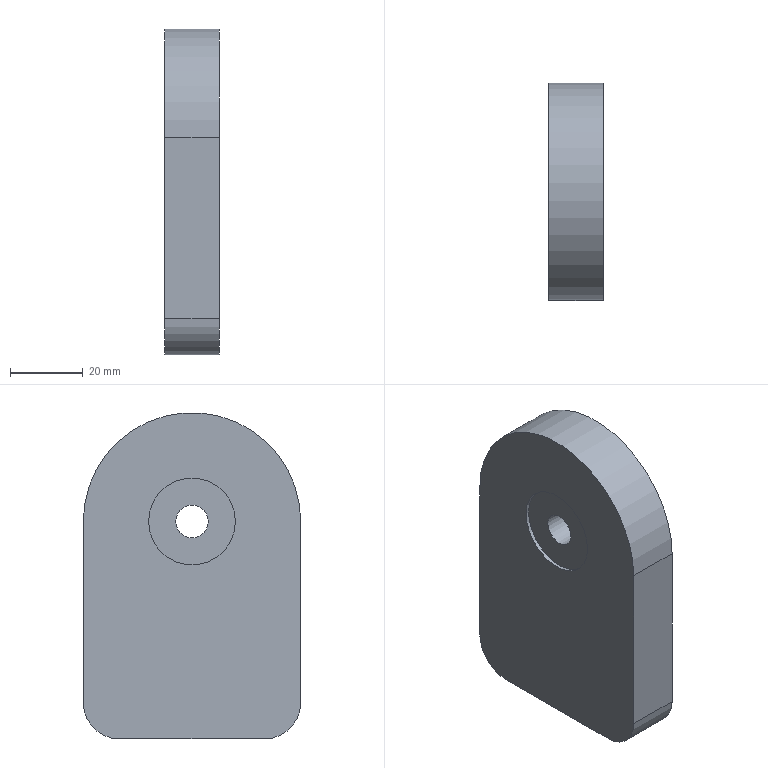Part | STEP file | Frame_lock | 1 solid | 11 faces | box 15 x 60 x 90 mm | volume 73219 mm3 | plane 6 | cylinder 5 | commonest cylinder face diameters 20 x2 9 x1 24 x1 60 x1
STEP:
#1=CARTESIAN_POINT('',(0.,0.,0.));
#2=DIRECTION('',(0.,0.,1.));
#3=DIRECTION('',(1.,0.,0.));
#4=AXIS2_PLACEMENT_3D('',#1,#2,#3);
#5=CARTESIAN_POINT('',(0.,30.,0.));
#6=VERTEX_POINT('',#5);
#7=CARTESIAN_POINT('',(0.,-30.,0.));
#8=VERTEX_POINT('',#7);
#9=CARTESIAN_POINT('',(0.,0.,0.));
#10=DIRECTION('',(1.,0.,0.));
#11=DIRECTION('',(0.,1.,0.));
#12=AXIS2_PLACEMENT_3D('',#9,#10,#11);
#13=CIRCLE('',#12,30.);
#14=CARTESIAN_POINT('',(0.,0.,0.));
#15=DIRECTION('',(-1.,0.,0.));
#16=DIRECTION('',(0.,1.,0.));
#17=AXIS2_PLACEMENT_3D('',#14,#15,#16);
#18=CYLINDRICAL_SURFACE('',#17,30.);
#19=CARTESIAN_POINT('',(6.283,0.));
#20=DIRECTION('',(-1.,0.));
#21=VECTOR('',#20,1.);
#22=LINE('',#19,#21);
#23=(GEOMETRIC_REPRESENTATION_CONTEXT(2)PARAMETRIC_REPRESENTATION_CONTEXT()REPRESENTATION_CONTEXT('',''));
#24=DEFINITIONAL_REPRESENTATION('',(#22),#23);
#25=PCURVE('',#18,#24);
#26=CARTESIAN_POINT('',(0.,0.,-17.885));
#27=DIRECTION('',(1.,0.,0.));
#28=DIRECTION('',(0.,0.,1.));
#29=AXIS2_PLACEMENT_3D('',#26,#27,#28);
#30=PLANE('',#29);
#31=CARTESIAN_POINT('',(17.885,0.));
#32=DIRECTION('',(0.,-1.));
#33=AXIS2_PLACEMENT_2D('',#31,#32);
#34=CIRCLE('',#33,30.);
#35=(GEOMETRIC_REPRESENTATION_CONTEXT(2)PARAMETRIC_REPRESENTATION_CONTEXT()REPRESENTATION_CONTEXT('',''));
#36=DEFINITIONAL_REPRESENTATION('',(#34),#35);
#37=PCURVE('',#30,#36);
#38=SURFACE_CURVE('',#13,(#25,#37),.PCURVE_S1.);
#39=EDGE_CURVE('',#6,#8,#38,.T.);
#40=ORIENTED_EDGE('',*,*,#39,.T.);
#41=CARTESIAN_POINT('',(15.,-30.,0.));
#42=VERTEX_POINT('',#41);
#43=CARTESIAN_POINT('',(0.,-30.,0.));
#44=DIRECTION('',(1.,0.,0.));
#45=VECTOR('',#44,1.);
#46=LINE('',#43,#45);
#47=CARTESIAN_POINT('',(3.142,0.));
#48=DIRECTION('',(0.,-1.));
#49=VECTOR('',#48,1.);
#50=LINE('',#47,#49);
#51=(GEOMETRIC_REPRESENTATION_CONTEXT(2)PARAMETRIC_REPRESENTATION_CONTEXT()REPRESENTATION_CONTEXT('',''));
#52=DEFINITIONAL_REPRESENTATION('',(#50),#51);
#53=PCURVE('',#18,#52);
#54=CARTESIAN_POINT('',(0.,-30.,0.));
#55=DIRECTION('',(0.,1.,0.));
#56=DIRECTION('',(0.,0.,-1.));
#57=AXIS2_PLACEMENT_3D('',#54,#55,#56);
#58=PLANE('',#57);
#59=CARTESIAN_POINT('',(0.,0.));
#60=DIRECTION('',(0.,-1.));
#61=VECTOR('',#60,1.);
#62=LINE('',#59,#61);
#63=(GEOMETRIC_REPRESENTATION_CONTEXT(2)PARAMETRIC_REPRESENTATION_CONTEXT()REPRESENTATION_CONTEXT('',''));
#64=DEFINITIONAL_REPRESENTATION('',(#62),#63);
#65=PCURVE('',#58,#64);
#66=SURFACE_CURVE('',#46,(#53,#65),.PCURVE_S1.);
#67=EDGE_CURVE('',#8,#42,#66,.T.);
#68=ORIENTED_EDGE('',*,*,#67,.T.);
#69=CARTESIAN_POINT('',(15.,30.,0.));
#70=VERTEX_POINT('',#69);
#71=CARTESIAN_POINT('',(15.,0.,0.));
#72=DIRECTION('',(1.,0.,0.));
#73=DIRECTION('',(0.,1.,0.));
#74=AXIS2_PLACEMENT_3D('',#71,#72,#73);
#75=CIRCLE('',#74,30.);
#76=CARTESIAN_POINT('',(6.283,-15.));
#77=DIRECTION('',(-1.,0.));
#78=VECTOR('',#77,1.);
#79=LINE('',#76,#78);
#80=(GEOMETRIC_REPRESENTATION_CONTEXT(2)PARAMETRIC_REPRESENTATION_CONTEXT()REPRESENTATION_CONTEXT('',''));
#81=DEFINITIONAL_REPRESENTATION('',(#79),#80);
#82=PCURVE('',#18,#81);
#83=CARTESIAN_POINT('',(15.,0.,-17.885));
#84=DIRECTION('',(1.,0.,0.));
#85=DIRECTION('',(0.,0.,1.));
#86=AXIS2_PLACEMENT_3D('',#83,#84,#85);
#87=PLANE('',#86);
#88=CARTESIAN_POINT('',(17.885,0.));
#89=DIRECTION('',(0.,-1.));
#90=AXIS2_PLACEMENT_2D('',#88,#89);
#91=CIRCLE('',#90,30.);
#92=(GEOMETRIC_REPRESENTATION_CONTEXT(2)PARAMETRIC_REPRESENTATION_CONTEXT()REPRESENTATION_CONTEXT('',''));
#93=DEFINITIONAL_REPRESENTATION('',(#91),#92);
#94=PCURVE('',#87,#93);
#95=SURFACE_CURVE('',#75,(#82,#94),.PCURVE_S1.);
#96=EDGE_CURVE('',#70,#42,#95,.T.);
#97=ORIENTED_EDGE('',*,*,#96,.F.);
#98=CARTESIAN_POINT('',(0.,30.,0.));
#99=DIRECTION('',(1.,0.,0.));
#100=VECTOR('',#99,1.);
#101=LINE('',#98,#100);
#102=CARTESIAN_POINT('',(6.283,0.));
#103=DIRECTION('',(0.,-1.));
#104=VECTOR('',#103,1.);
#105=LINE('',#102,#104);
#106=(GEOMETRIC_REPRESENTATION_CONTEXT(2)PARAMETRIC_REPRESENTATION_CONTEXT()REPRESENTATION_CONTEXT('',''));
#107=DEFINITIONAL_REPRESENTATION('',(#105),#106);
#108=PCURVE('',#18,#107);
#109=CARTESIAN_POINT('',(0.,30.,-50.));
#110=DIRECTION('',(0.,-1.,0.));
#111=DIRECTION('',(0.,0.,1.));
#112=AXIS2_PLACEMENT_3D('',#109,#110,#111);
#113=PLANE('',#112);
#114=CARTESIAN_POINT('',(50.,0.));
#115=DIRECTION('',(0.,-1.));
#116=VECTOR('',#115,1.);
#117=LINE('',#114,#116);
#118=(GEOMETRIC_REPRESENTATION_CONTEXT(2)PARAMETRIC_REPRESENTATION_CONTEXT()REPRESENTATION_CONTEXT('',''));
#119=DEFINITIONAL_REPRESENTATION('',(#117),#118);
#120=PCURVE('',#113,#119);
#121=SURFACE_CURVE('',#101,(#108,#120),.PCURVE_S1.);
#122=EDGE_CURVE('',#6,#70,#121,.T.);
#123=ORIENTED_EDGE('',*,*,#122,.F.);
#124=EDGE_LOOP('',(#40,#68,#97,#123));
#125=FACE_BOUND('',#124,.T.);
#126=ADVANCED_FACE('',(#125),#18,.T.);
#127=CARTESIAN_POINT('',(0.,30.,-50.));
#128=VERTEX_POINT('',#127);
#129=CARTESIAN_POINT('',(15.,30.,-50.));
#130=VERTEX_POINT('',#129);
#131=CARTESIAN_POINT('',(0.,30.,-50.));
#132=DIRECTION('',(1.,0.,0.));
#133=VECTOR('',#132,1.);
#134=LINE('',#131,#133);
#135=CARTESIAN_POINT('',(0.,0.));
#136=DIRECTION('',(0.,-1.));
#137=VECTOR('',#136,1.);
#138=LINE('',#135,#137);
#139=(GEOMETRIC_REPRESENTATION_CONTEXT(2)PARAMETRIC_REPRESENTATION_CONTEXT()REPRESENTATION_CONTEXT('',''));
#140=DEFINITIONAL_REPRESENTATION('',(#138),#139);
#141=PCURVE('',#113,#140);
#142=CARTESIAN_POINT('',(0.,20.,-50.));
#143=DIRECTION('',(-1.,0.,0.));
#144=DIRECTION('',(0.,1.,0.));
#145=AXIS2_PLACEMENT_3D('',#142,#143,#144);
#146=CYLINDRICAL_SURFACE('',#145,10.);
#147=CARTESIAN_POINT('',(0.,0.));
#148=DIRECTION('',(0.,-1.));
#149=VECTOR('',#148,1.);
#150=LINE('',#147,#149);
#151=(GEOMETRIC_REPRESENTATION_CONTEXT(2)PARAMETRIC_REPRESENTATION_CONTEXT()REPRESENTATION_CONTEXT('',''));
#152=DEFINITIONAL_REPRESENTATION('',(#150),#151);
#153=PCURVE('',#146,#152);
#154=SURFACE_CURVE('',#134,(#141,#153),.PCURVE_S1.);
#155=EDGE_CURVE('',#128,#130,#154,.T.);
#156=ORIENTED_EDGE('',*,*,#155,.T.);
#157=CARTESIAN_POINT('',(15.,30.,-50.));
#158=DIRECTION('',(0.,0.,1.));
#159=VECTOR('',#158,1.);
#160=LINE('',#157,#159);
#161=CARTESIAN_POINT('',(0.,-15.));
#162=DIRECTION('',(1.,0.));
#163=VECTOR('',#162,1.);
#164=LINE('',#161,#163);
#165=(GEOMETRIC_REPRESENTATION_CONTEXT(2)PARAMETRIC_REPRESENTATION_CONTEXT()REPRESENTATION_CONTEXT('',''));
#166=DEFINITIONAL_REPRESENTATION('',(#164),#165);
#167=PCURVE('',#113,#166);
#168=CARTESIAN_POINT('',(-32.115,-30.));
#169=DIRECTION('',(1.,0.));
#170=VECTOR('',#169,1.);
#171=LINE('',#168,#170);
#172=(GEOMETRIC_REPRESENTATION_CONTEXT(2)PARAMETRIC_REPRESENTATION_CONTEXT()REPRESENTATION_CONTEXT('',''));
#173=DEFINITIONAL_REPRESENTATION('',(#171),#172);
#174=PCURVE('',#87,#173);
#175=SURFACE_CURVE('',#160,(#167,#174),.PCURVE_S1.);
#176=EDGE_CURVE('',#130,#70,#175,.T.);
#177=ORIENTED_EDGE('',*,*,#176,.T.);
#178=ORIENTED_EDGE('',*,*,#122,.F.);
#179=CARTESIAN_POINT('',(0.,30.,-50.));
#180=DIRECTION('',(0.,0.,1.));
#181=VECTOR('',#180,1.);
#182=LINE('',#179,#181);
#183=CARTESIAN_POINT('',(0.,0.));
#184=DIRECTION('',(1.,0.));
#185=VECTOR('',#184,1.);
#186=LINE('',#183,#185);
#187=(GEOMETRIC_REPRESENTATION_CONTEXT(2)PARAMETRIC_REPRESENTATION_CONTEXT()REPRESENTATION_CONTEXT('',''));
#188=DEFINITIONAL_REPRESENTATION('',(#186),#187);
#189=PCURVE('',#113,#188);
#190=CARTESIAN_POINT('',(-32.115,-30.));
#191=DIRECTION('',(1.,0.));
#192=VECTOR('',#191,1.);
#193=LINE('',#190,#192);
#194=(GEOMETRIC_REPRESENTATION_CONTEXT(2)PARAMETRIC_REPRESENTATION_CONTEXT()REPRESENTATION_CONTEXT('',''));
#195=DEFINITIONAL_REPRESENTATION('',(#193),#194);
#196=PCURVE('',#30,#195);
#197=SURFACE_CURVE('',#182,(#189,#196),.PCURVE_S1.);
#198=EDGE_CURVE('',#128,#6,#197,.T.);
#199=ORIENTED_EDGE('',*,*,#198,.F.);
#200=EDGE_LOOP('',(#156,#177,#178,#199));
#201=FACE_BOUND('',#200,.F.);
#202=ADVANCED_FACE('',(#201),#113,.F.);
#203=ORIENTED_EDGE('',*,*,#67,.T.);
#204=CARTESIAN_POINT('',(15.,-30.,-50.));
#205=VERTEX_POINT('',#204);
#206=CARTESIAN_POINT('',(15.,-30.,0.));
#207=DIRECTION('',(0.,0.,-1.));
#208=VECTOR('',#207,1.);
#209=LINE('',#206,#208);
#210=CARTESIAN_POINT('',(0.,-15.));
#211=DIRECTION('',(1.,0.));
#212=VECTOR('',#211,1.);
#213=LINE('',#210,#212);
#214=(GEOMETRIC_REPRESENTATION_CONTEXT(2)PARAMETRIC_REPRESENTATION_CONTEXT()REPRESENTATION_CONTEXT('',''));
#215=DEFINITIONAL_REPRESENTATION('',(#213),#214);
#216=PCURVE('',#58,#215);
#217=CARTESIAN_POINT('',(17.885,30.));
#218=DIRECTION('',(-1.,0.));
#219=VECTOR('',#218,1.);
#220=LINE('',#217,#219);
#221=(GEOMETRIC_REPRESENTATION_CONTEXT(2)PARAMETRIC_REPRESENTATION_CONTEXT()REPRESENTATION_CONTEXT('',''));
#222=DEFINITIONAL_REPRESENTATION('',(#220),#221);
#223=PCURVE('',#87,#222);
#224=SURFACE_CURVE('',#209,(#216,#223),.PCURVE_S1.);
#225=EDGE_CURVE('',#42,#205,#224,.T.);
#226=ORIENTED_EDGE('',*,*,#225,.T.);
#227=CARTESIAN_POINT('',(0.,-30.,-50.));
#228=VERTEX_POINT('',#227);
#229=CARTESIAN_POINT('',(0.,-30.,-50.));
#230=DIRECTION('',(1.,0.,0.));
#231=VECTOR('',#230,1.);
#232=LINE('',#229,#231);
#233=CARTESIAN_POINT('',(50.,0.));
#234=DIRECTION('',(0.,-1.));
#235=VECTOR('',#234,1.);
#236=LINE('',#233,#235);
#237=(GEOMETRIC_REPRESENTATION_CONTEXT(2)PARAMETRIC_REPRESENTATION_CONTEXT()REPRESENTATION_CONTEXT('',''));
#238=DEFINITIONAL_REPRESENTATION('',(#236),#237);
#239=PCURVE('',#58,#238);
#240=CARTESIAN_POINT('',(0.,-20.,-50.));
#241=DIRECTION('',(-1.,0.,0.));
#242=DIRECTION('',(0.,1.,0.));
#243=AXIS2_PLACEMENT_3D('',#240,#241,#242);
#244=CYLINDRICAL_SURFACE('',#243,10.);
#245=CARTESIAN_POINT('',(3.142,0.));
#246=DIRECTION('',(0.,-1.));
#247=VECTOR('',#246,1.);
#248=LINE('',#245,#247);
#249=(GEOMETRIC_REPRESENTATION_CONTEXT(2)PARAMETRIC_REPRESENTATION_CONTEXT()REPRESENTATION_CONTEXT('',''));
#250=DEFINITIONAL_REPRESENTATION('',(#248),#249);
#251=PCURVE('',#244,#250);
#252=SURFACE_CURVE('',#232,(#239,#251),.PCURVE_S1.);
#253=EDGE_CURVE('',#228,#205,#252,.T.);
#254=ORIENTED_EDGE('',*,*,#253,.F.);
#255=CARTESIAN_POINT('',(0.,-30.,0.));
#256=DIRECTION('',(0.,0.,-1.));
#257=VECTOR('',#256,1.);
#258=LINE('',#255,#257);
#259=CARTESIAN_POINT('',(0.,0.));
#260=DIRECTION('',(1.,0.));
#261=VECTOR('',#260,1.);
#262=LINE('',#259,#261);
#263=(GEOMETRIC_REPRESENTATION_CONTEXT(2)PARAMETRIC_REPRESENTATION_CONTEXT()REPRESENTATION_CONTEXT('',''));
#264=DEFINITIONAL_REPRESENTATION('',(#262),#263);
#265=PCURVE('',#58,#264);
#266=CARTESIAN_POINT('',(17.885,30.));
#267=DIRECTION('',(-1.,0.));
#268=VECTOR('',#267,1.);
#269=LINE('',#266,#268);
#270=(GEOMETRIC_REPRESENTATION_CONTEXT(2)PARAMETRIC_REPRESENTATION_CONTEXT()REPRESENTATION_CONTEXT('',''));
#271=DEFINITIONAL_REPRESENTATION('',(#269),#270);
#272=PCURVE('',#30,#271);
#273=SURFACE_CURVE('',#258,(#265,#272),.PCURVE_S1.);
#274=EDGE_CURVE('',#8,#228,#273,.T.);
#275=ORIENTED_EDGE('',*,*,#274,.F.);
#276=EDGE_LOOP('',(#203,#226,#254,#275));
#277=FACE_BOUND('',#276,.F.);
#278=ADVANCED_FACE('',(#277),#58,.F.);
#279=ORIENTED_EDGE('',*,*,#39,.T.);
#280=ORIENTED_EDGE('',*,*,#274,.T.);
#281=CARTESIAN_POINT('',(0.,-20.,-60.));
#282=VERTEX_POINT('',#281);
#283=CARTESIAN_POINT('',(0.,-20.,-50.));
#284=DIRECTION('',(1.,0.,0.));
#285=DIRECTION('',(0.,1.,0.));
#286=AXIS2_PLACEMENT_3D('',#283,#284,#285);
#287=CIRCLE('',#286,10.);
#288=CARTESIAN_POINT('',(-32.115,20.));
#289=DIRECTION('',(0.,-1.));
#290=AXIS2_PLACEMENT_2D('',#288,#289);
#291=CIRCLE('',#290,10.);
#292=(GEOMETRIC_REPRESENTATION_CONTEXT(2)PARAMETRIC_REPRESENTATION_CONTEXT()REPRESENTATION_CONTEXT('',''));
#293=DEFINITIONAL_REPRESENTATION('',(#291),#292);
#294=PCURVE('',#30,#293);
#295=CARTESIAN_POINT('',(6.283,0.));
#296=DIRECTION('',(-1.,0.));
#297=VECTOR('',#296,1.);
#298=LINE('',#295,#297);
#299=(GEOMETRIC_REPRESENTATION_CONTEXT(2)PARAMETRIC_REPRESENTATION_CONTEXT()REPRESENTATION_CONTEXT('',''));
#300=DEFINITIONAL_REPRESENTATION('',(#298),#299);
#301=PCURVE('',#244,#300);
#302=SURFACE_CURVE('',#287,(#294,#301),.PCURVE_S1.);
#303=EDGE_CURVE('',#228,#282,#302,.T.);
#304=ORIENTED_EDGE('',*,*,#303,.T.);
#305=CARTESIAN_POINT('',(0.,20.,-60.));
#306=VERTEX_POINT('',#305);
#307=CARTESIAN_POINT('',(0.,-20.,-60.));
#308=DIRECTION('',(0.,1.,0.));
#309=VECTOR('',#308,1.);
#310=LINE('',#307,#309);
#311=CARTESIAN_POINT('',(-42.115,20.));
#312=DIRECTION('',(0.,-1.));
#313=VECTOR('',#312,1.);
#314=LINE('',#311,#313);
#315=(GEOMETRIC_REPRESENTATION_CONTEXT(2)PARAMETRIC_REPRESENTATION_CONTEXT()REPRESENTATION_CONTEXT('',''));
#316=DEFINITIONAL_REPRESENTATION('',(#314),#315);
#317=PCURVE('',#30,#316);
#318=CARTESIAN_POINT('',(0.,-20.,-60.));
#319=DIRECTION('',(0.,0.,1.));
#320=DIRECTION('',(0.,1.,0.));
#321=AXIS2_PLACEMENT_3D('',#318,#319,#320);
#322=PLANE('',#321);
#323=CARTESIAN_POINT('',(0.,0.));
#324=DIRECTION('',(1.,0.));
#325=VECTOR('',#324,1.);
#326=LINE('',#323,#325);
#327=(GEOMETRIC_REPRESENTATION_CONTEXT(2)PARAMETRIC_REPRESENTATION_CONTEXT()REPRESENTATION_CONTEXT('',''));
#328=DEFINITIONAL_REPRESENTATION('',(#326),#327);
#329=PCURVE('',#322,#328);
#330=SURFACE_CURVE('',#310,(#317,#329),.PCURVE_S1.);
#331=EDGE_CURVE('',#282,#306,#330,.T.);
#332=ORIENTED_EDGE('',*,*,#331,.T.);
#333=CARTESIAN_POINT('',(0.,20.,-50.));
#334=DIRECTION('',(1.,0.,0.));
#335=DIRECTION('',(0.,1.,0.));
#336=AXIS2_PLACEMENT_3D('',#333,#334,#335);
#337=CIRCLE('',#336,10.);
#338=CARTESIAN_POINT('',(-32.115,-20.));
#339=DIRECTION('',(0.,-1.));
#340=AXIS2_PLACEMENT_2D('',#338,#339);
#341=CIRCLE('',#340,10.);
#342=(GEOMETRIC_REPRESENTATION_CONTEXT(2)PARAMETRIC_REPRESENTATION_CONTEXT()REPRESENTATION_CONTEXT('',''));
#343=DEFINITIONAL_REPRESENTATION('',(#341),#342);
#344=PCURVE('',#30,#343);
#345=CARTESIAN_POINT('',(6.283,0.));
#346=DIRECTION('',(-1.,0.));
#347=VECTOR('',#346,1.);
#348=LINE('',#345,#347);
#349=(GEOMETRIC_REPRESENTATION_CONTEXT(2)PARAMETRIC_REPRESENTATION_CONTEXT()REPRESENTATION_CONTEXT('',''));
#350=DEFINITIONAL_REPRESENTATION('',(#348),#349);
#351=PCURVE('',#146,#350);
#352=SURFACE_CURVE('',#337,(#344,#351),.PCURVE_S1.);
#353=EDGE_CURVE('',#306,#128,#352,.T.);
#354=ORIENTED_EDGE('',*,*,#353,.T.);
#355=ORIENTED_EDGE('',*,*,#198,.T.);
#356=EDGE_LOOP('',(#279,#280,#304,#332,#354,#355));
#357=FACE_BOUND('',#356,.F.);
#358=CARTESIAN_POINT('',(0.,-12.,0.));
#359=VERTEX_POINT('',#358);
#360=CARTESIAN_POINT('',(0.,0.,0.));
#361=DIRECTION('',(-1.,0.,0.));
#362=DIRECTION('',(0.,-1.,0.));
#363=AXIS2_PLACEMENT_3D('',#360,#361,#362);
#364=CIRCLE('',#363,12.);
#365=CARTESIAN_POINT('',(17.885,12.));
#366=CARTESIAN_POINT('',(38.67,12.));
#367=CARTESIAN_POINT('',(28.277,-6.));
#368=CARTESIAN_POINT('',(17.885,-24.));
#369=CARTESIAN_POINT('',(7.493,-6.));
#370=CARTESIAN_POINT('',(-2.9,12.));
#371=CARTESIAN_POINT('',(17.885,12.));
#372=(BOUNDED_CURVE()B_SPLINE_CURVE(2,(#365,#366,#367,#368,#369,#370,#371),.UNSPECIFIED.,.T.,.F.)B_SPLINE_CURVE_WITH_KNOTS((1,2,2,2,2,1),(-2.094,0.,2.094,4.189,6.283,8.378),.UNSPECIFIED.)CURVE()GEOMETRIC_REPRESENTATION_ITEM()RATIONAL_B_SPLINE_CURVE((1.,0.5,1.,0.5,1.,0.5,1.))REPRESENTATION_ITEM(''));
#373=(GEOMETRIC_REPRESENTATION_CONTEXT(2)PARAMETRIC_REPRESENTATION_CONTEXT()REPRESENTATION_CONTEXT('',''));
#374=DEFINITIONAL_REPRESENTATION('',(#372),#373);
#375=PCURVE('',#30,#374);
#376=CARTESIAN_POINT('',(0.,0.,0.));
#377=DIRECTION('',(-1.,0.,0.));
#378=DIRECTION('',(0.,-1.,0.));
#379=AXIS2_PLACEMENT_3D('',#376,#377,#378);
#380=CYLINDRICAL_SURFACE('',#379,12.);
#381=CARTESIAN_POINT('',(0.,0.));
#382=DIRECTION('',(1.,0.));
#383=VECTOR('',#382,1.);
#384=LINE('',#381,#383);
#385=(GEOMETRIC_REPRESENTATION_CONTEXT(2)PARAMETRIC_REPRESENTATION_CONTEXT()REPRESENTATION_CONTEXT('',''));
#386=DEFINITIONAL_REPRESENTATION('',(#384),#385);
#387=PCURVE('',#380,#386);
#388=SURFACE_CURVE('',#364,(#375,#387),.PCURVE_S1.);
#389=EDGE_CURVE('',#359,#359,#388,.T.);
#390=ORIENTED_EDGE('',*,*,#389,.T.);
#391=EDGE_LOOP('',(#390));
#392=FACE_BOUND('',#391,.F.);
#393=ADVANCED_FACE('',(#357,#392),#30,.F.);
#394=ORIENTED_EDGE('',*,*,#96,.T.);
#395=ORIENTED_EDGE('',*,*,#225,.T.);
#396=CARTESIAN_POINT('',(15.,-20.,-60.));
#397=VERTEX_POINT('',#396);
#398=CARTESIAN_POINT('',(15.,-20.,-50.));
#399=DIRECTION('',(1.,0.,0.));
#400=DIRECTION('',(0.,1.,0.));
#401=AXIS2_PLACEMENT_3D('',#398,#399,#400);
#402=CIRCLE('',#401,10.);
#403=CARTESIAN_POINT('',(-32.115,20.));
#404=DIRECTION('',(0.,-1.));
#405=AXIS2_PLACEMENT_2D('',#403,#404);
#406=CIRCLE('',#405,10.);
#407=(GEOMETRIC_REPRESENTATION_CONTEXT(2)PARAMETRIC_REPRESENTATION_CONTEXT()REPRESENTATION_CONTEXT('',''));
#408=DEFINITIONAL_REPRESENTATION('',(#406),#407);
#409=PCURVE('',#87,#408);
#410=CARTESIAN_POINT('',(6.283,-15.));
#411=DIRECTION('',(-1.,0.));
#412=VECTOR('',#411,1.);
#413=LINE('',#410,#412);
#414=(GEOMETRIC_REPRESENTATION_CONTEXT(2)PARAMETRIC_REPRESENTATION_CONTEXT()REPRESENTATION_CONTEXT('',''));
#415=DEFINITIONAL_REPRESENTATION('',(#413),#414);
#416=PCURVE('',#244,#415);
#417=SURFACE_CURVE('',#402,(#409,#416),.PCURVE_S1.);
#418=EDGE_CURVE('',#205,#397,#417,.T.);
#419=ORIENTED_EDGE('',*,*,#418,.T.);
#420=CARTESIAN_POINT('',(15.,20.,-60.));
#421=VERTEX_POINT('',#420);
#422=CARTESIAN_POINT('',(15.,-20.,-60.));
#423=DIRECTION('',(0.,1.,0.));
#424=VECTOR('',#423,1.);
#425=LINE('',#422,#424);
#426=CARTESIAN_POINT('',(-42.115,20.));
#427=DIRECTION('',(0.,-1.));
#428=VECTOR('',#427,1.);
#429=LINE('',#426,#428);
#430=(GEOMETRIC_REPRESENTATION_CONTEXT(2)PARAMETRIC_REPRESENTATION_CONTEXT()REPRESENTATION_CONTEXT('',''));
#431=DEFINITIONAL_REPRESENTATION('',(#429),#430);
#432=PCURVE('',#87,#431);
#433=CARTESIAN_POINT('',(0.,-15.));
#434=DIRECTION('',(1.,0.));
#435=VECTOR('',#434,1.);
#436=LINE('',#433,#435);
#437=(GEOMETRIC_REPRESENTATION_CONTEXT(2)PARAMETRIC_REPRESENTATION_CONTEXT()REPRESENTATION_CONTEXT('',''));
#438=DEFINITIONAL_REPRESENTATION('',(#436),#437);
#439=PCURVE('',#322,#438);
#440=SURFACE_CURVE('',#425,(#432,#439),.PCURVE_S1.);
#441=EDGE_CURVE('',#397,#421,#440,.T.);
#442=ORIENTED_EDGE('',*,*,#441,.T.);
#443=CARTESIAN_POINT('',(15.,20.,-50.));
#444=DIRECTION('',(1.,0.,0.));
#445=DIRECTION('',(0.,1.,0.));
#446=AXIS2_PLACEMENT_3D('',#443,#444,#445);
#447=CIRCLE('',#446,10.);
#448=CARTESIAN_POINT('',(-32.115,-20.));
#449=DIRECTION('',(0.,-1.));
#450=AXIS2_PLACEMENT_2D('',#448,#449);
#451=CIRCLE('',#450,10.);
#452=(GEOMETRIC_REPRESENTATION_CONTEXT(2)PARAMETRIC_REPRESENTATION_CONTEXT()REPRESENTATION_CONTEXT('',''));
#453=DEFINITIONAL_REPRESENTATION('',(#451),#452);
#454=PCURVE('',#87,#453);
#455=CARTESIAN_POINT('',(6.283,-15.));
#456=DIRECTION('',(-1.,0.));
#457=VECTOR('',#456,1.);
#458=LINE('',#455,#457);
#459=(GEOMETRIC_REPRESENTATION_CONTEXT(2)PARAMETRIC_REPRESENTATION_CONTEXT()REPRESENTATION_CONTEXT('',''));
#460=DEFINITIONAL_REPRESENTATION('',(#458),#459);
#461=PCURVE('',#146,#460);
#462=SURFACE_CURVE('',#447,(#454,#461),.PCURVE_S1.);
#463=EDGE_CURVE('',#421,#130,#462,.T.);
#464=ORIENTED_EDGE('',*,*,#463,.T.);
#465=ORIENTED_EDGE('',*,*,#176,.T.);
#466=EDGE_LOOP('',(#394,#395,#419,#442,#464,#465));
#467=FACE_BOUND('',#466,.T.);
#468=CARTESIAN_POINT('',(15.,4.5,0.));
#469=VERTEX_POINT('',#468);
#470=CARTESIAN_POINT('',(15.,0.,0.));
#471=DIRECTION('',(1.,0.,0.));
#472=DIRECTION('',(0.,1.,0.));
#473=AXIS2_PLACEMENT_3D('',#470,#471,#472);
#474=CIRCLE('',#473,4.5);
#475=CARTESIAN_POINT('',(17.885,0.));
#476=DIRECTION('',(0.,-1.));
#477=AXIS2_PLACEMENT_2D('',#475,#476);
#478=CIRCLE('',#477,4.5);
#479=(GEOMETRIC_REPRESENTATION_CONTEXT(2)PARAMETRIC_REPRESENTATION_CONTEXT()REPRESENTATION_CONTEXT('',''));
#480=DEFINITIONAL_REPRESENTATION('',(#478),#479);
#481=PCURVE('',#87,#480);
#482=CARTESIAN_POINT('',(0.,0.,0.));
#483=DIRECTION('',(-1.,0.,0.));
#484=DIRECTION('',(0.,1.,0.));
#485=AXIS2_PLACEMENT_3D('',#482,#483,#484);
#486=CYLINDRICAL_SURFACE('',#485,4.5);
#487=CARTESIAN_POINT('',(6.283,-15.));
#488=DIRECTION('',(-1.,0.));
#489=VECTOR('',#488,1.);
#490=LINE('',#487,#489);
#491=(GEOMETRIC_REPRESENTATION_CONTEXT(2)PARAMETRIC_REPRESENTATION_CONTEXT()REPRESENTATION_CONTEXT('',''));
#492=DEFINITIONAL_REPRESENTATION('',(#490),#491);
#493=PCURVE('',#486,#492);
#494=SURFACE_CURVE('',#474,(#481,#493),.PCURVE_S1.);
#495=EDGE_CURVE('',#469,#469,#494,.T.);
#496=ORIENTED_EDGE('',*,*,#495,.T.);
#497=EDGE_LOOP('',(#496));
#498=FACE_BOUND('',#497,.F.);
#499=ADVANCED_FACE('',(#467,#498),#87,.T.);
#500=ORIENTED_EDGE('',*,*,#353,.T.);
#501=ORIENTED_EDGE('',*,*,#155,.T.);
#502=ORIENTED_EDGE('',*,*,#463,.F.);
#503=CARTESIAN_POINT('',(0.,20.,-60.));
#504=DIRECTION('',(1.,0.,0.));
#505=VECTOR('',#504,1.);
#506=LINE('',#503,#505);
#507=CARTESIAN_POINT('',(1.571,0.));
#508=DIRECTION('',(0.,-1.));
#509=VECTOR('',#508,1.);
#510=LINE('',#507,#509);
#511=(GEOMETRIC_REPRESENTATION_CONTEXT(2)PARAMETRIC_REPRESENTATION_CONTEXT()REPRESENTATION_CONTEXT('',''));
#512=DEFINITIONAL_REPRESENTATION('',(#510),#511);
#513=PCURVE('',#146,#512);
#514=CARTESIAN_POINT('',(40.,0.));
#515=DIRECTION('',(0.,-1.));
#516=VECTOR('',#515,1.);
#517=LINE('',#514,#516);
#518=(GEOMETRIC_REPRESENTATION_CONTEXT(2)PARAMETRIC_REPRESENTATION_CONTEXT()REPRESENTATION_CONTEXT('',''));
#519=DEFINITIONAL_REPRESENTATION('',(#517),#518);
#520=PCURVE('',#322,#519);
#521=SURFACE_CURVE('',#506,(#513,#520),.PCURVE_S1.);
#522=EDGE_CURVE('',#306,#421,#521,.T.);
#523=ORIENTED_EDGE('',*,*,#522,.F.);
#524=EDGE_LOOP('',(#500,#501,#502,#523));
#525=FACE_BOUND('',#524,.T.);
#526=ADVANCED_FACE('',(#525),#146,.T.);
#527=ORIENTED_EDGE('',*,*,#303,.T.);
#528=CARTESIAN_POINT('',(0.,-20.,-60.));
#529=DIRECTION('',(1.,0.,0.));
#530=VECTOR('',#529,1.);
#531=LINE('',#528,#530);
#532=CARTESIAN_POINT('',(1.571,0.));
#533=DIRECTION('',(0.,-1.));
#534=VECTOR('',#533,1.);
#535=LINE('',#532,#534);
#536=(GEOMETRIC_REPRESENTATION_CONTEXT(2)PARAMETRIC_REPRESENTATION_CONTEXT()REPRESENTATION_CONTEXT('',''));
#537=DEFINITIONAL_REPRESENTATION('',(#535),#536);
#538=PCURVE('',#244,#537);
#539=CARTESIAN_POINT('',(0.,0.));
#540=DIRECTION('',(0.,-1.));
#541=VECTOR('',#540,1.);
#542=LINE('',#539,#541);
#543=(GEOMETRIC_REPRESENTATION_CONTEXT(2)PARAMETRIC_REPRESENTATION_CONTEXT()REPRESENTATION_CONTEXT('',''));
#544=DEFINITIONAL_REPRESENTATION('',(#542),#543);
#545=PCURVE('',#322,#544);
#546=SURFACE_CURVE('',#531,(#538,#545),.PCURVE_S1.);
#547=EDGE_CURVE('',#282,#397,#546,.T.);
#548=ORIENTED_EDGE('',*,*,#547,.T.);
#549=ORIENTED_EDGE('',*,*,#418,.F.);
#550=ORIENTED_EDGE('',*,*,#253,.F.);
#551=EDGE_LOOP('',(#527,#548,#549,#550));
#552=FACE_BOUND('',#551,.T.);
#553=ADVANCED_FACE('',(#552),#244,.T.);
#554=ORIENTED_EDGE('',*,*,#547,.T.);
#555=ORIENTED_EDGE('',*,*,#441,.T.);
#556=ORIENTED_EDGE('',*,*,#522,.F.);
#557=ORIENTED_EDGE('',*,*,#331,.F.);
#558=EDGE_LOOP('',(#554,#555,#556,#557));
#559=FACE_BOUND('',#558,.F.);
#560=ADVANCED_FACE('',(#559),#322,.F.);
#561=CARTESIAN_POINT('',(1.,-12.,0.));
#562=VERTEX_POINT('',#561);
#563=CARTESIAN_POINT('',(0.,-12.,0.));
#564=DIRECTION('',(1.,0.,0.));
#565=VECTOR('',#564,1.);
#566=LINE('',#563,#565);
#567=CARTESIAN_POINT('',(0.,0.));
#568=DIRECTION('',(0.,-1.));
#569=VECTOR('',#568,1.);
#570=LINE('',#567,#569);
#571=(GEOMETRIC_REPRESENTATION_CONTEXT(2)PARAMETRIC_REPRESENTATION_CONTEXT()REPRESENTATION_CONTEXT('',''));
#572=DEFINITIONAL_REPRESENTATION('',(#570),#571);
#573=PCURVE('',#380,#572);
#574=CARTESIAN_POINT('',(6.283,0.));
#575=DIRECTION('',(0.,-1.));
#576=VECTOR('',#575,1.);
#577=LINE('',#574,#576);
#578=(GEOMETRIC_REPRESENTATION_CONTEXT(2)PARAMETRIC_REPRESENTATION_CONTEXT()REPRESENTATION_CONTEXT('',''));
#579=DEFINITIONAL_REPRESENTATION('',(#577),#578);
#580=PCURVE('',#380,#579);
#581=SEAM_CURVE('',#566,(#573,#580),.PCURVE_S1.);
#582=EDGE_CURVE('',#359,#562,#581,.T.);
#583=ORIENTED_EDGE('',*,*,#582,.T.);
#584=CARTESIAN_POINT('',(1.,0.,0.));
#585=DIRECTION('',(-1.,0.,0.));
#586=DIRECTION('',(0.,-1.,0.));
#587=AXIS2_PLACEMENT_3D('',#584,#585,#586);
#588=CIRCLE('',#587,12.);
#589=CARTESIAN_POINT('',(0.,-1.));
#590=DIRECTION('',(1.,0.));
#591=VECTOR('',#590,1.);
#592=LINE('',#589,#591);
#593=(GEOMETRIC_REPRESENTATION_CONTEXT(2)PARAMETRIC_REPRESENTATION_CONTEXT()REPRESENTATION_CONTEXT('',''));
#594=DEFINITIONAL_REPRESENTATION('',(#592),#593);
#595=PCURVE('',#380,#594);
#596=CARTESIAN_POINT('',(1.,0.,0.));
#597=DIRECTION('',(1.,0.,0.));
#598=DIRECTION('',(0.,0.,1.));
#599=AXIS2_PLACEMENT_3D('',#596,#597,#598);
#600=PLANE('',#599);
#601=CARTESIAN_POINT('',(0.,12.));
#602=CARTESIAN_POINT('',(20.785,12.));
#603=CARTESIAN_POINT('',(10.392,-6.));
#604=CARTESIAN_POINT('',(0.,-24.));
#605=CARTESIAN_POINT('',(-10.392,-6.));
#606=CARTESIAN_POINT('',(-20.785,12.));
#607=CARTESIAN_POINT('',(0.,12.));
#608=(BOUNDED_CURVE()B_SPLINE_CURVE(2,(#601,#602,#603,#604,#605,#606,#607),.UNSPECIFIED.,.T.,.F.)B_SPLINE_CURVE_WITH_KNOTS((1,2,2,2,2,1),(-2.094,0.,2.094,4.189,6.283,8.378),.UNSPECIFIED.)CURVE()GEOMETRIC_REPRESENTATION_ITEM()RATIONAL_B_SPLINE_CURVE((1.,0.5,1.,0.5,1.,0.5,1.))REPRESENTATION_ITEM(''));
#609=(GEOMETRIC_REPRESENTATION_CONTEXT(2)PARAMETRIC_REPRESENTATION_CONTEXT()REPRESENTATION_CONTEXT('',''));
#610=DEFINITIONAL_REPRESENTATION('',(#608),#609);
#611=PCURVE('',#600,#610);
#612=SURFACE_CURVE('',#588,(#595,#611),.PCURVE_S1.);
#613=EDGE_CURVE('',#562,#562,#612,.T.);
#614=ORIENTED_EDGE('',*,*,#613,.T.);
#615=ORIENTED_EDGE('',*,*,#582,.F.);
#616=ORIENTED_EDGE('',*,*,#389,.F.);
#617=EDGE_LOOP('',(#583,#614,#615,#616));
#618=FACE_BOUND('',#617,.F.);
#619=ADVANCED_FACE('',(#618),#380,.F.);
#620=CARTESIAN_POINT('',(1.,4.5,0.));
#621=VERTEX_POINT('',#620);
#622=CARTESIAN_POINT('',(0.,4.5,0.));
#623=DIRECTION('',(1.,0.,0.));
#624=VECTOR('',#623,1.);
#625=LINE('',#622,#624);
#626=CARTESIAN_POINT('',(0.,0.));
#627=DIRECTION('',(0.,-1.));
#628=VECTOR('',#627,1.);
#629=LINE('',#626,#628);
#630=(GEOMETRIC_REPRESENTATION_CONTEXT(2)PARAMETRIC_REPRESENTATION_CONTEXT()REPRESENTATION_CONTEXT('',''));
#631=DEFINITIONAL_REPRESENTATION('',(#629),#630);
#632=PCURVE('',#486,#631);
#633=CARTESIAN_POINT('',(6.283,0.));
#634=DIRECTION('',(0.,-1.));
#635=VECTOR('',#634,1.);
#636=LINE('',#633,#635);
#637=(GEOMETRIC_REPRESENTATION_CONTEXT(2)PARAMETRIC_REPRESENTATION_CONTEXT()REPRESENTATION_CONTEXT('',''));
#638=DEFINITIONAL_REPRESENTATION('',(#636),#637);
#639=PCURVE('',#486,#638);
#640=SEAM_CURVE('',#625,(#632,#639),.PCURVE_S1.);
#641=EDGE_CURVE('',#621,#469,#640,.T.);
#642=ORIENTED_EDGE('',*,*,#641,.T.);
#643=ORIENTED_EDGE('',*,*,#495,.F.);
#644=ORIENTED_EDGE('',*,*,#641,.F.);
#645=CARTESIAN_POINT('',(1.,0.,0.));
#646=DIRECTION('',(-1.,0.,0.));
#647=DIRECTION('',(0.,1.,0.));
#648=AXIS2_PLACEMENT_3D('',#645,#646,#647);
#649=CIRCLE('',#648,4.5);
#650=CARTESIAN_POINT('',(0.,-1.));
#651=DIRECTION('',(1.,0.));
#652=VECTOR('',#651,1.);
#653=LINE('',#650,#652);
#654=(GEOMETRIC_REPRESENTATION_CONTEXT(2)PARAMETRIC_REPRESENTATION_CONTEXT()REPRESENTATION_CONTEXT('',''));
#655=DEFINITIONAL_REPRESENTATION('',(#653),#654);
#656=PCURVE('',#486,#655);
#657=CARTESIAN_POINT('',(0.,-4.5));
#658=CARTESIAN_POINT('',(-7.794,-4.5));
#659=CARTESIAN_POINT('',(-3.897,2.25));
#660=CARTESIAN_POINT('',(0.,9.));
#661=CARTESIAN_POINT('',(3.897,2.25));
#662=CARTESIAN_POINT('',(7.794,-4.5));
#663=CARTESIAN_POINT('',(0.,-4.5));
#664=(BOUNDED_CURVE()B_SPLINE_CURVE(2,(#657,#658,#659,#660,#661,#662,#663),.UNSPECIFIED.,.T.,.F.)B_SPLINE_CURVE_WITH_KNOTS((1,2,2,2,2,1),(-2.094,0.,2.094,4.189,6.283,8.378),.UNSPECIFIED.)CURVE()GEOMETRIC_REPRESENTATION_ITEM()RATIONAL_B_SPLINE_CURVE((1.,0.5,1.,0.5,1.,0.5,1.))REPRESENTATION_ITEM(''));
#665=(GEOMETRIC_REPRESENTATION_CONTEXT(2)PARAMETRIC_REPRESENTATION_CONTEXT()REPRESENTATION_CONTEXT('',''));
#666=DEFINITIONAL_REPRESENTATION('',(#664),#665);
#667=PCURVE('',#600,#666);
#668=SURFACE_CURVE('',#649,(#656,#667),.PCURVE_S1.);
#669=EDGE_CURVE('',#621,#621,#668,.T.);
#670=ORIENTED_EDGE('',*,*,#669,.F.);
#671=EDGE_LOOP('',(#642,#643,#644,#670));
#672=FACE_BOUND('',#671,.F.);
#673=ADVANCED_FACE('',(#672),#486,.F.);
#674=ORIENTED_EDGE('',*,*,#613,.F.);
#675=EDGE_LOOP('',(#674));
#676=FACE_BOUND('',#675,.F.);
#677=ORIENTED_EDGE('',*,*,#669,.T.);
#678=EDGE_LOOP('',(#677));
#679=FACE_BOUND('',#678,.F.);
#680=ADVANCED_FACE('',(#676,#679),#600,.F.);
#681=CLOSED_SHELL('',(#126,#202,#278,#393,#499,#526,#553,#560,#619,#673,#680));
#682=MANIFOLD_SOLID_BREP('',#681);
#683=(LENGTH_UNIT()NAMED_UNIT(*)SI_UNIT(.MILLI.,.METRE.));
#684=UNCERTAINTY_MEASURE_WITH_UNIT(LENGTH_MEASURE(0.0000001),#683,'','');
#685=(NAMED_UNIT(*)PLANE_ANGLE_UNIT()SI_UNIT($,.RADIAN.));
#686=(NAMED_UNIT(*)SI_UNIT($,.STERADIAN.)SOLID_ANGLE_UNIT());
#687=(GEOMETRIC_REPRESENTATION_CONTEXT(3)GLOBAL_UNCERTAINTY_ASSIGNED_CONTEXT((#684))GLOBAL_UNIT_ASSIGNED_CONTEXT((#683,#685,#686))REPRESENTATION_CONTEXT('',''));
#688=ADVANCED_BREP_SHAPE_REPRESENTATION('',(#4,#682),#687);